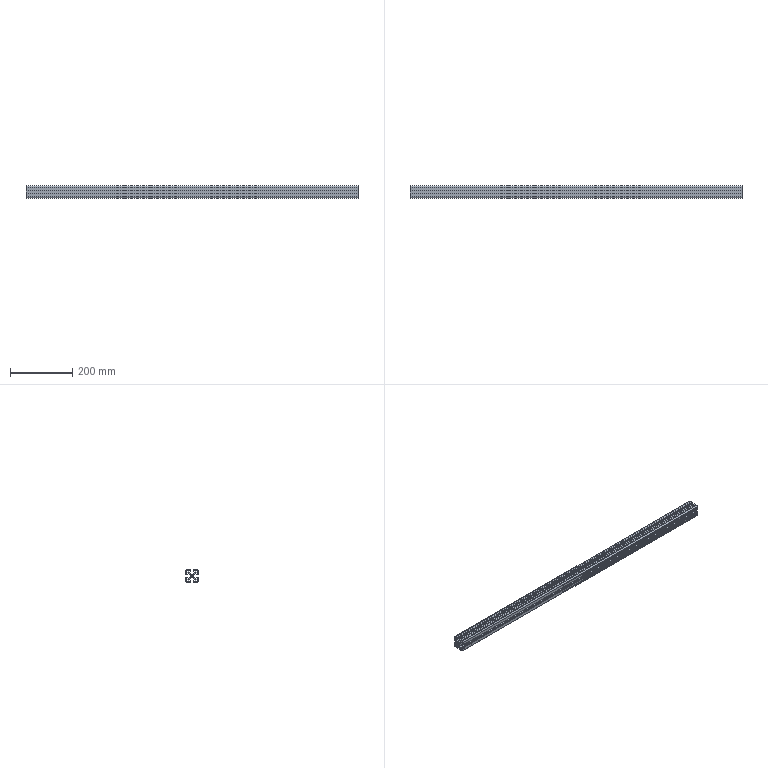Part | STEP file | 1 solid | 188 faces | box 1070 x 40 x 40 mm | volume 511726 mm3 | cylinder 94 | plane 94 | commonest cylinder face diameters 0.6 x30 2 x28 4 x16 0.4 x8 6 x4 9 x4